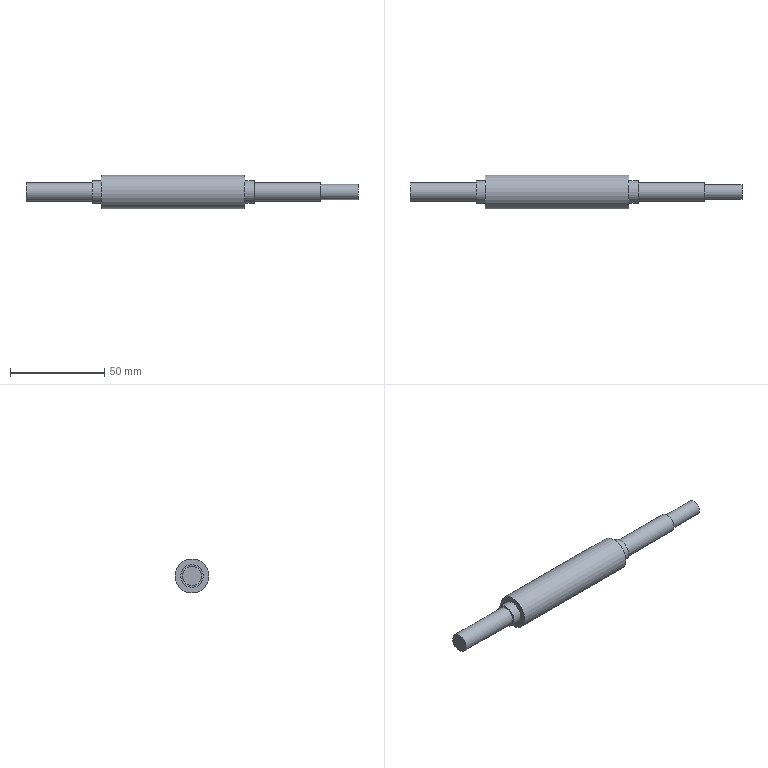Part | NX | 1 solid | 13 faces | box 176 x 18 x 18 mm | volume 26974 mm3 | plane 7 | cylinder 6 | commonest cylinder face diameters 10 x2 12 x2 8 x1 18 x1
STEP:
#1=CARTESIAN_POINT('',(78.,0.,-5.));
#2=VERTEX_POINT('',#1);
#3=CARTESIAN_POINT('',(78.,0.,0.));
#4=DIRECTION('',(1.,0.,0.));
#5=DIRECTION('',(0.,0.,-1.));
#6=AXIS2_PLACEMENT_3D('',#3,#4,#5);
#7=CIRCLE('',#6,5.);
#8=EDGE_CURVE('',#2,#2,#7,.T.);
#9=ORIENTED_EDGE('',*,*,#8,.T.);
#10=EDGE_LOOP('',(#9));
#11=FACE_BOUND('',#10,.T.);
#12=CARTESIAN_POINT('',(78.,0.,-4.));
#13=VERTEX_POINT('',#12);
#14=CARTESIAN_POINT('',(78.,0.,0.));
#15=DIRECTION('',(1.,0.,0.));
#16=DIRECTION('',(0.,0.,-1.));
#17=AXIS2_PLACEMENT_3D('',#14,#15,#16);
#18=CIRCLE('',#17,4.);
#19=EDGE_CURVE('',#13,#13,#18,.T.);
#20=ORIENTED_EDGE('',*,*,#19,.F.);
#21=EDGE_LOOP('',(#20));
#22=FACE_BOUND('',#21,.T.);
#23=CARTESIAN_POINT('',(78.,0.,0.));
#24=DIRECTION('',(1.,0.,0.));
#25=DIRECTION('',(0.,0.,-1.));
#26=AXIS2_PLACEMENT_3D('',#23,#24,#25);
#27=PLANE('',#26);
#28=ADVANCED_FACE('',(#11,#22),#27,.T.);
#29=CARTESIAN_POINT('',(43.,0.,-6.));
#30=VERTEX_POINT('',#29);
#31=CARTESIAN_POINT('',(43.,0.,0.));
#32=DIRECTION('',(1.,0.,0.));
#33=DIRECTION('',(0.,0.,-1.));
#34=AXIS2_PLACEMENT_3D('',#31,#32,#33);
#35=CIRCLE('',#34,6.);
#36=EDGE_CURVE('',#30,#30,#35,.T.);
#37=ORIENTED_EDGE('',*,*,#36,.T.);
#38=EDGE_LOOP('',(#37));
#39=FACE_BOUND('',#38,.T.);
#40=CARTESIAN_POINT('',(43.,0.,-5.));
#41=VERTEX_POINT('',#40);
#42=CARTESIAN_POINT('',(43.,0.,0.));
#43=DIRECTION('',(1.,0.,0.));
#44=DIRECTION('',(0.,0.,-1.));
#45=AXIS2_PLACEMENT_3D('',#42,#43,#44);
#46=CIRCLE('',#45,5.);
#47=EDGE_CURVE('',#41,#41,#46,.T.);
#48=ORIENTED_EDGE('',*,*,#47,.F.);
#49=EDGE_LOOP('',(#48));
#50=FACE_BOUND('',#49,.T.);
#51=CARTESIAN_POINT('',(43.,0.,0.));
#52=DIRECTION('',(1.,0.,0.));
#53=DIRECTION('',(0.,0.,-1.));
#54=AXIS2_PLACEMENT_3D('',#51,#52,#53);
#55=PLANE('',#54);
#56=ADVANCED_FACE('',(#39,#50),#55,.T.);
#57=CARTESIAN_POINT('',(38.,0.,-9.));
#58=VERTEX_POINT('',#57);
#59=CARTESIAN_POINT('',(38.,0.,0.));
#60=DIRECTION('',(1.,0.,0.));
#61=DIRECTION('',(0.,0.,-1.));
#62=AXIS2_PLACEMENT_3D('',#59,#60,#61);
#63=CIRCLE('',#62,9.);
#64=EDGE_CURVE('',#58,#58,#63,.T.);
#65=ORIENTED_EDGE('',*,*,#64,.T.);
#66=EDGE_LOOP('',(#65));
#67=FACE_BOUND('',#66,.T.);
#68=CARTESIAN_POINT('',(38.,0.,-6.));
#69=VERTEX_POINT('',#68);
#70=CARTESIAN_POINT('',(38.,0.,0.));
#71=DIRECTION('',(1.,0.,0.));
#72=DIRECTION('',(0.,0.,-1.));
#73=AXIS2_PLACEMENT_3D('',#70,#71,#72);
#74=CIRCLE('',#73,6.);
#75=EDGE_CURVE('',#69,#69,#74,.T.);
#76=ORIENTED_EDGE('',*,*,#75,.F.);
#77=EDGE_LOOP('',(#76));
#78=FACE_BOUND('',#77,.T.);
#79=CARTESIAN_POINT('',(38.,0.,0.));
#80=DIRECTION('',(1.,0.,0.));
#81=DIRECTION('',(0.,0.,-1.));
#82=AXIS2_PLACEMENT_3D('',#79,#80,#81);
#83=PLANE('',#82);
#84=ADVANCED_FACE('',(#67,#78),#83,.T.);
#85=ORIENTED_EDGE('',*,*,#64,.F.);
#86=EDGE_LOOP('',(#85));
#87=FACE_BOUND('',#86,.T.);
#88=CARTESIAN_POINT('',(-38.,0.,-9.));
#89=VERTEX_POINT('',#88);
#90=CARTESIAN_POINT('',(-38.,0.,0.));
#91=DIRECTION('',(1.,0.,0.));
#92=DIRECTION('',(0.,0.,-1.));
#93=AXIS2_PLACEMENT_3D('',#90,#91,#92);
#94=CIRCLE('',#93,9.);
#95=EDGE_CURVE('',#89,#89,#94,.T.);
#96=ORIENTED_EDGE('',*,*,#95,.T.);
#97=EDGE_LOOP('',(#96));
#98=FACE_BOUND('',#97,.T.);
#99=CARTESIAN_POINT('',(38.,0.,0.));
#100=DIRECTION('',(-1.,0.,0.));
#101=DIRECTION('',(0.,0.,1.));
#102=AXIS2_PLACEMENT_3D('',#99,#100,#101);
#103=CYLINDRICAL_SURFACE('',#102,9.);
#104=ADVANCED_FACE('',(#87,#98),#103,.T.);
#105=CARTESIAN_POINT('',(-38.,0.,-6.));
#106=VERTEX_POINT('',#105);
#107=CARTESIAN_POINT('',(-38.,0.,0.));
#108=DIRECTION('',(1.,0.,0.));
#109=DIRECTION('',(0.,0.,-1.));
#110=AXIS2_PLACEMENT_3D('',#107,#108,#109);
#111=CIRCLE('',#110,6.);
#112=EDGE_CURVE('',#106,#106,#111,.T.);
#113=ORIENTED_EDGE('',*,*,#112,.T.);
#114=EDGE_LOOP('',(#113));
#115=FACE_BOUND('',#114,.T.);
#116=ORIENTED_EDGE('',*,*,#95,.F.);
#117=EDGE_LOOP('',(#116));
#118=FACE_BOUND('',#117,.T.);
#119=CARTESIAN_POINT('',(-38.,0.,0.));
#120=DIRECTION('',(1.,0.,0.));
#121=DIRECTION('',(0.,0.,-1.));
#122=AXIS2_PLACEMENT_3D('',#119,#120,#121);
#123=PLANE('',#122);
#124=ADVANCED_FACE('',(#115,#118),#123,.F.);
#125=ORIENTED_EDGE('',*,*,#36,.F.);
#126=EDGE_LOOP('',(#125));
#127=FACE_BOUND('',#126,.T.);
#128=ORIENTED_EDGE('',*,*,#75,.T.);
#129=EDGE_LOOP('',(#128));
#130=FACE_BOUND('',#129,.T.);
#131=CARTESIAN_POINT('',(43.,0.,0.));
#132=DIRECTION('',(-1.,0.,0.));
#133=DIRECTION('',(0.,0.,1.));
#134=AXIS2_PLACEMENT_3D('',#131,#132,#133);
#135=CYLINDRICAL_SURFACE('',#134,6.);
#136=ADVANCED_FACE('',(#127,#130),#135,.T.);
#137=ORIENTED_EDGE('',*,*,#8,.F.);
#138=EDGE_LOOP('',(#137));
#139=FACE_BOUND('',#138,.T.);
#140=ORIENTED_EDGE('',*,*,#47,.T.);
#141=EDGE_LOOP('',(#140));
#142=FACE_BOUND('',#141,.T.);
#143=CARTESIAN_POINT('',(78.,0.,0.));
#144=DIRECTION('',(-1.,0.,0.));
#145=DIRECTION('',(0.,0.,1.));
#146=AXIS2_PLACEMENT_3D('',#143,#144,#145);
#147=CYLINDRICAL_SURFACE('',#146,5.);
#148=ADVANCED_FACE('',(#139,#142),#147,.T.);
#149=CARTESIAN_POINT('',(98.,0.,-4.));
#150=VERTEX_POINT('',#149);
#151=CARTESIAN_POINT('',(98.,0.,0.));
#152=DIRECTION('',(1.,0.,0.));
#153=DIRECTION('',(0.,0.,-1.));
#154=AXIS2_PLACEMENT_3D('',#151,#152,#153);
#155=CIRCLE('',#154,4.);
#156=EDGE_CURVE('',#150,#150,#155,.T.);
#157=ORIENTED_EDGE('',*,*,#156,.F.);
#158=EDGE_LOOP('',(#157));
#159=FACE_BOUND('',#158,.T.);
#160=ORIENTED_EDGE('',*,*,#19,.T.);
#161=EDGE_LOOP('',(#160));
#162=FACE_BOUND('',#161,.T.);
#163=CARTESIAN_POINT('',(98.,0.,0.));
#164=DIRECTION('',(-1.,0.,0.));
#165=DIRECTION('',(0.,0.,1.));
#166=AXIS2_PLACEMENT_3D('',#163,#164,#165);
#167=CYLINDRICAL_SURFACE('',#166,4.);
#168=ADVANCED_FACE('',(#159,#162),#167,.T.);
#169=ORIENTED_EDGE('',*,*,#156,.T.);
#170=EDGE_LOOP('',(#169));
#171=FACE_BOUND('',#170,.T.);
#172=CARTESIAN_POINT('',(98.,0.,0.));
#173=DIRECTION('',(1.,0.,0.));
#174=DIRECTION('',(0.,0.,-1.));
#175=AXIS2_PLACEMENT_3D('',#172,#173,#174);
#176=PLANE('',#175);
#177=ADVANCED_FACE('',(#171),#176,.T.);
#178=CARTESIAN_POINT('',(-43.,0.,-6.));
#179=VERTEX_POINT('',#178);
#180=CARTESIAN_POINT('',(-43.,0.,0.));
#181=DIRECTION('',(1.,0.,0.));
#182=DIRECTION('',(0.,0.,-1.));
#183=AXIS2_PLACEMENT_3D('',#180,#181,#182);
#184=CIRCLE('',#183,6.);
#185=EDGE_CURVE('',#179,#179,#184,.T.);
#186=ORIENTED_EDGE('',*,*,#185,.T.);
#187=EDGE_LOOP('',(#186));
#188=FACE_BOUND('',#187,.T.);
#189=ORIENTED_EDGE('',*,*,#112,.F.);
#190=EDGE_LOOP('',(#189));
#191=FACE_BOUND('',#190,.T.);
#192=CARTESIAN_POINT('',(-43.,0.,0.));
#193=DIRECTION('',(1.,0.,0.));
#194=DIRECTION('',(0.,0.,-1.));
#195=AXIS2_PLACEMENT_3D('',#192,#193,#194);
#196=CYLINDRICAL_SURFACE('',#195,6.);
#197=ADVANCED_FACE('',(#188,#191),#196,.T.);
#198=CARTESIAN_POINT('',(-43.,0.,5.));
#199=VERTEX_POINT('',#198);
#200=CARTESIAN_POINT('',(-43.,0.,0.));
#201=DIRECTION('',(-1.,0.,0.));
#202=DIRECTION('',(0.,0.,1.));
#203=AXIS2_PLACEMENT_3D('',#200,#201,#202);
#204=CIRCLE('',#203,5.);
#205=EDGE_CURVE('',#199,#199,#204,.T.);
#206=ORIENTED_EDGE('',*,*,#205,.F.);
#207=EDGE_LOOP('',(#206));
#208=FACE_BOUND('',#207,.T.);
#209=ORIENTED_EDGE('',*,*,#185,.F.);
#210=EDGE_LOOP('',(#209));
#211=FACE_BOUND('',#210,.T.);
#212=CARTESIAN_POINT('',(-43.,0.,0.));
#213=DIRECTION('',(-1.,0.,0.));
#214=DIRECTION('',(0.,0.,-1.));
#215=AXIS2_PLACEMENT_3D('',#212,#213,#214);
#216=PLANE('',#215);
#217=ADVANCED_FACE('',(#208,#211),#216,.T.);
#218=CARTESIAN_POINT('',(-78.,0.,-5.));
#219=VERTEX_POINT('',#218);
#220=CARTESIAN_POINT('',(-78.,0.,0.));
#221=DIRECTION('',(1.,0.,0.));
#222=DIRECTION('',(0.,0.,-1.));
#223=AXIS2_PLACEMENT_3D('',#220,#221,#222);
#224=CIRCLE('',#223,5.);
#225=EDGE_CURVE('',#219,#219,#224,.T.);
#226=ORIENTED_EDGE('',*,*,#225,.T.);
#227=EDGE_LOOP('',(#226));
#228=FACE_BOUND('',#227,.T.);
#229=ORIENTED_EDGE('',*,*,#205,.T.);
#230=EDGE_LOOP('',(#229));
#231=FACE_BOUND('',#230,.T.);
#232=CARTESIAN_POINT('',(-78.,0.,0.));
#233=DIRECTION('',(1.,0.,0.));
#234=DIRECTION('',(0.,0.,-1.));
#235=AXIS2_PLACEMENT_3D('',#232,#233,#234);
#236=CYLINDRICAL_SURFACE('',#235,5.);
#237=ADVANCED_FACE('',(#228,#231),#236,.T.);
#238=ORIENTED_EDGE('',*,*,#225,.F.);
#239=EDGE_LOOP('',(#238));
#240=FACE_BOUND('',#239,.T.);
#241=CARTESIAN_POINT('',(-78.,0.,0.));
#242=DIRECTION('',(-1.,0.,0.));
#243=DIRECTION('',(0.,0.,-1.));
#244=AXIS2_PLACEMENT_3D('',#241,#242,#243);
#245=PLANE('',#244);
#246=ADVANCED_FACE('',(#240),#245,.T.);
#247=CLOSED_SHELL('',(#28,#56,#84,#104,#124,#136,#148,#168,#177,#197,#217,#237,#246));
#248=MANIFOLD_SOLID_BREP('',#247);
#249=(LENGTH_UNIT()NAMED_UNIT(*)SI_UNIT(.MILLI.,.METRE.));
#250=UNCERTAINTY_MEASURE_WITH_UNIT(LENGTH_MEASURE(0.00001),#249,'','');
#251=(NAMED_UNIT(*)PLANE_ANGLE_UNIT()SI_UNIT($,.RADIAN.));
#252=(NAMED_UNIT(*)SI_UNIT($,.STERADIAN.)SOLID_ANGLE_UNIT());
#253=(GEOMETRIC_REPRESENTATION_CONTEXT(3)GLOBAL_UNCERTAINTY_ASSIGNED_CONTEXT((#250))GLOBAL_UNIT_ASSIGNED_CONTEXT((#249,#251,#252))REPRESENTATION_CONTEXT('',''));
#254=ADVANCED_BREP_SHAPE_REPRESENTATION('',(#248),#253);